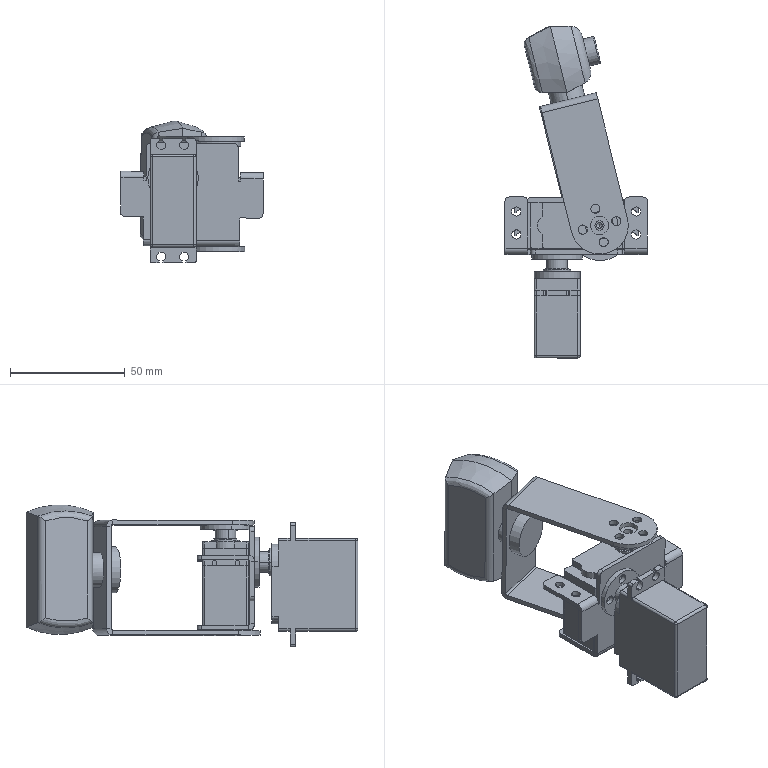Part | SolidWorks | features MirrorCompFeat 1 | 6 solids | 400 faces | box 62.179 x 144.352 x 61.763 mm | volume 114357 mm3 | cylinder 204 | plane 170 | cone 10 | sphere 10 | torus 6 | commonest cylinder face diameters 4 x74 2 x36 5.8 x20 5 x18 8 x8 10 x8